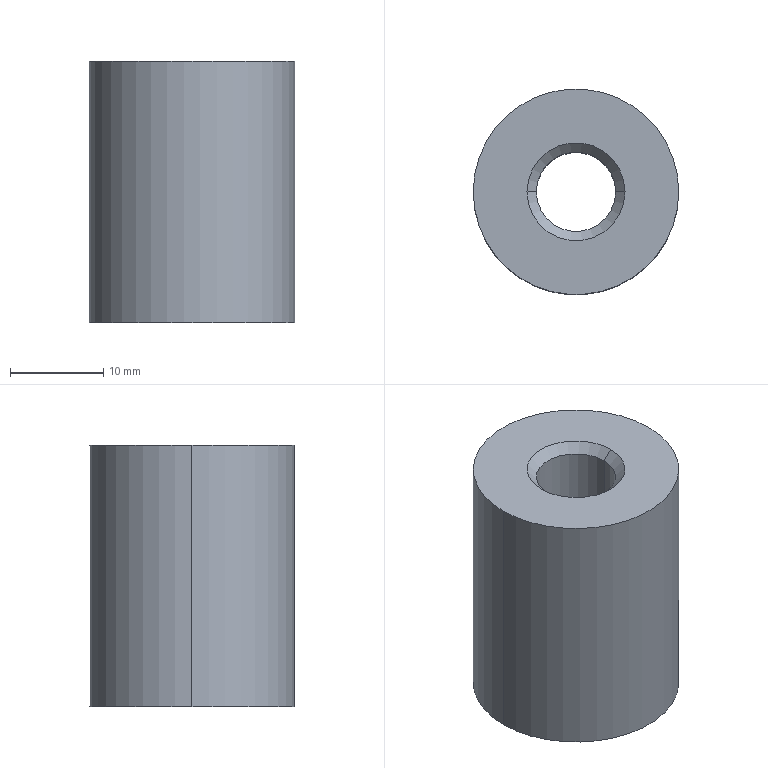Part | SolidWorks | features Chamfer 1, Extrusion 1, Helix 1, ICE 1 | 1 solid | 8 faces | box 22 x 22 x 28 mm | volume 9040 mm3 | cylinder 4 | cone 2 | plane 2 | commonest cylinder face diameters 8.5 x2 22 x2
STEP:
#1=CARTESIAN_POINT('',(-4.25,0.,27.));
#2=VERTEX_POINT('',#1);
#3=CARTESIAN_POINT('',(4.25,0.,27.));
#4=VERTEX_POINT('',#3);
#5=CARTESIAN_POINT('',(0.,0.,27.));
#6=DIRECTION('',(0.,0.,1.));
#7=DIRECTION('',(1.,0.,0.));
#8=AXIS2_PLACEMENT_3D('',#5,#6,#7);
#9=CIRCLE('',#8,4.25);
#10=EDGE_CURVE('',#2,#4,#9,.T.);
#11=ORIENTED_EDGE('',*,*,#10,.F.);
#12=CARTESIAN_POINT('',(-5.25,0.,28.));
#13=VERTEX_POINT('',#12);
#14=CARTESIAN_POINT('',(-4.25,0.,27.));
#15=DIRECTION('',(-0.7071,0.,0.7071));
#16=VECTOR('',#15,1000.);
#17=LINE('',#14,#16);
#18=EDGE_CURVE('',#2,#13,#17,.T.);
#19=ORIENTED_EDGE('',*,*,#18,.T.);
#20=CARTESIAN_POINT('',(5.25,0.,28.));
#21=VERTEX_POINT('',#20);
#22=CARTESIAN_POINT('',(0.,0.,28.));
#23=DIRECTION('',(0.,0.,-1.));
#24=DIRECTION('',(1.,0.,0.));
#25=AXIS2_PLACEMENT_3D('',#22,#23,#24);
#26=CIRCLE('',#25,5.25);
#27=EDGE_CURVE('',#21,#13,#26,.T.);
#28=ORIENTED_EDGE('',*,*,#27,.F.);
#29=CARTESIAN_POINT('',(4.25,0.,27.));
#30=DIRECTION('',(0.7071,0.,0.7071));
#31=VECTOR('',#30,1000.);
#32=LINE('',#29,#31);
#33=EDGE_CURVE('',#4,#21,#32,.T.);
#34=ORIENTED_EDGE('',*,*,#33,.F.);
#35=EDGE_LOOP('',(#11,#19,#28,#34));
#36=FACE_OUTER_BOUND('',#35,.T.);
#37=CARTESIAN_POINT('',(0.,0.,27.));
#38=DIRECTION('',(0.,0.,1.));
#39=DIRECTION('',(1.,0.,0.));
#40=AXIS2_PLACEMENT_3D('',#37,#38,#39);
#41=CONICAL_SURFACE('',#40,4.25,0.7854);
#42=ADVANCED_FACE('',(#36),#41,.F.);
#43=CARTESIAN_POINT('',(-4.25,0.,0.));
#44=VERTEX_POINT('',#43);
#45=CARTESIAN_POINT('',(4.25,0.,0.));
#46=VERTEX_POINT('',#45);
#47=CARTESIAN_POINT('',(0.,0.,0.));
#48=DIRECTION('',(0.,0.,1.));
#49=DIRECTION('',(1.,0.,0.));
#50=AXIS2_PLACEMENT_3D('',#47,#48,#49);
#51=CIRCLE('',#50,4.25);
#52=EDGE_CURVE('',#44,#46,#51,.T.);
#53=ORIENTED_EDGE('',*,*,#52,.F.);
#54=CARTESIAN_POINT('',(-4.25,0.,-10.));
#55=DIRECTION('',(0.,0.,1.));
#56=VECTOR('',#55,1000.);
#57=LINE('',#54,#56);
#58=EDGE_CURVE('',#44,#2,#57,.T.);
#59=ORIENTED_EDGE('',*,*,#58,.T.);
#60=ORIENTED_EDGE('',*,*,#10,.T.);
#61=CARTESIAN_POINT('',(4.25,0.,-10.));
#62=DIRECTION('',(0.,0.,1.));
#63=VECTOR('',#62,1000.);
#64=LINE('',#61,#63);
#65=EDGE_CURVE('',#46,#4,#64,.T.);
#66=ORIENTED_EDGE('',*,*,#65,.F.);
#67=EDGE_LOOP('',(#53,#59,#60,#66));
#68=FACE_OUTER_BOUND('',#67,.T.);
#69=CARTESIAN_POINT('',(0.,0.,-10.));
#70=DIRECTION('',(0.,0.,1.));
#71=DIRECTION('',(1.,0.,0.));
#72=AXIS2_PLACEMENT_3D('',#69,#70,#71);
#73=CYLINDRICAL_SURFACE('',#72,4.25);
#74=ADVANCED_FACE('',(#68),#73,.F.);
#75=CARTESIAN_POINT('',(11.,0.,28.));
#76=VERTEX_POINT('',#75);
#77=CARTESIAN_POINT('',(-11.,0.,28.));
#78=VERTEX_POINT('',#77);
#79=CARTESIAN_POINT('',(0.,0.,28.));
#80=DIRECTION('',(0.,0.,1.));
#81=DIRECTION('',(1.,0.,0.));
#82=AXIS2_PLACEMENT_3D('',#79,#80,#81);
#83=CIRCLE('',#82,11.);
#84=EDGE_CURVE('',#76,#78,#83,.T.);
#85=ORIENTED_EDGE('',*,*,#84,.F.);
#86=CARTESIAN_POINT('',(11.,0.,0.));
#87=VERTEX_POINT('',#86);
#88=CARTESIAN_POINT('',(11.,0.,28.));
#89=DIRECTION('',(0.,0.,-1.));
#90=VECTOR('',#89,1000.);
#91=LINE('',#88,#90);
#92=EDGE_CURVE('',#76,#87,#91,.T.);
#93=ORIENTED_EDGE('',*,*,#92,.T.);
#94=CARTESIAN_POINT('',(-11.,0.,0.));
#95=VERTEX_POINT('',#94);
#96=CARTESIAN_POINT('',(0.,0.,0.));
#97=DIRECTION('',(0.,0.,1.));
#98=DIRECTION('',(1.,0.,0.));
#99=AXIS2_PLACEMENT_3D('',#96,#97,#98);
#100=CIRCLE('',#99,11.);
#101=EDGE_CURVE('',#87,#95,#100,.T.);
#102=ORIENTED_EDGE('',*,*,#101,.T.);
#103=CARTESIAN_POINT('',(-11.,0.,28.));
#104=DIRECTION('',(0.,0.,-1.));
#105=VECTOR('',#104,1000.);
#106=LINE('',#103,#105);
#107=EDGE_CURVE('',#78,#95,#106,.T.);
#108=ORIENTED_EDGE('',*,*,#107,.F.);
#109=EDGE_LOOP('',(#85,#93,#102,#108));
#110=FACE_OUTER_BOUND('',#109,.T.);
#111=CARTESIAN_POINT('',(0.,0.,28.));
#112=DIRECTION('',(0.,0.,-1.));
#113=DIRECTION('',(-1.,0.,0.));
#114=AXIS2_PLACEMENT_3D('',#111,#112,#113);
#115=CYLINDRICAL_SURFACE('',#114,11.);
#116=ADVANCED_FACE('',(#110),#115,.T.);
#117=ORIENTED_EDGE('',*,*,#92,.F.);
#118=CARTESIAN_POINT('',(0.,0.,28.));
#119=DIRECTION('',(0.,0.,1.));
#120=DIRECTION('',(1.,0.,0.));
#121=AXIS2_PLACEMENT_3D('',#118,#119,#120);
#122=CIRCLE('',#121,11.);
#123=EDGE_CURVE('',#78,#76,#122,.T.);
#124=ORIENTED_EDGE('',*,*,#123,.F.);
#125=ORIENTED_EDGE('',*,*,#107,.T.);
#126=CARTESIAN_POINT('',(0.,0.,0.));
#127=DIRECTION('',(0.,0.,1.));
#128=DIRECTION('',(1.,0.,0.));
#129=AXIS2_PLACEMENT_3D('',#126,#127,#128);
#130=CIRCLE('',#129,11.);
#131=EDGE_CURVE('',#95,#87,#130,.T.);
#132=ORIENTED_EDGE('',*,*,#131,.T.);
#133=EDGE_LOOP('',(#117,#124,#125,#132));
#134=FACE_OUTER_BOUND('',#133,.T.);
#135=CARTESIAN_POINT('',(0.,0.,28.));
#136=DIRECTION('',(0.,0.,-1.));
#137=DIRECTION('',(-1.,0.,0.));
#138=AXIS2_PLACEMENT_3D('',#135,#136,#137);
#139=CYLINDRICAL_SURFACE('',#138,11.);
#140=ADVANCED_FACE('',(#134),#139,.T.);
#141=ORIENTED_EDGE('',*,*,#27,.T.);
#142=CARTESIAN_POINT('',(0.,0.,28.));
#143=DIRECTION('',(0.,0.,-1.));
#144=DIRECTION('',(1.,0.,0.));
#145=AXIS2_PLACEMENT_3D('',#142,#143,#144);
#146=CIRCLE('',#145,5.25);
#147=EDGE_CURVE('',#13,#21,#146,.T.);
#148=ORIENTED_EDGE('',*,*,#147,.T.);
#149=EDGE_LOOP('',(#141,#148));
#150=FACE_BOUND('',#149,.T.);
#151=ORIENTED_EDGE('',*,*,#123,.T.);
#152=ORIENTED_EDGE('',*,*,#84,.T.);
#153=EDGE_LOOP('',(#151,#152));
#154=FACE_OUTER_BOUND('',#153,.T.);
#155=CARTESIAN_POINT('',(0.,0.,28.));
#156=DIRECTION('',(0.,0.,1.));
#157=DIRECTION('',(1.,0.,0.));
#158=AXIS2_PLACEMENT_3D('',#155,#156,#157);
#159=PLANE('',#158);
#160=ADVANCED_FACE('',(#150,#154),#159,.T.);
#161=CARTESIAN_POINT('',(0.,0.,0.));
#162=DIRECTION('',(0.,0.,1.));
#163=DIRECTION('',(1.,0.,0.));
#164=AXIS2_PLACEMENT_3D('',#161,#162,#163);
#165=CIRCLE('',#164,4.25);
#166=EDGE_CURVE('',#46,#44,#165,.T.);
#167=ORIENTED_EDGE('',*,*,#166,.T.);
#168=ORIENTED_EDGE('',*,*,#52,.T.);
#169=EDGE_LOOP('',(#167,#168));
#170=FACE_BOUND('',#169,.T.);
#171=ORIENTED_EDGE('',*,*,#131,.F.);
#172=ORIENTED_EDGE('',*,*,#101,.F.);
#173=EDGE_LOOP('',(#171,#172));
#174=FACE_OUTER_BOUND('',#173,.T.);
#175=CARTESIAN_POINT('',(0.,0.,0.));
#176=DIRECTION('',(0.,0.,1.));
#177=DIRECTION('',(1.,0.,0.));
#178=AXIS2_PLACEMENT_3D('',#175,#176,#177);
#179=PLANE('',#178);
#180=ADVANCED_FACE('',(#170,#174),#179,.F.);
#181=ORIENTED_EDGE('',*,*,#58,.F.);
#182=ORIENTED_EDGE('',*,*,#166,.F.);
#183=ORIENTED_EDGE('',*,*,#65,.T.);
#184=CARTESIAN_POINT('',(0.,0.,27.));
#185=DIRECTION('',(0.,0.,1.));
#186=DIRECTION('',(1.,0.,0.));
#187=AXIS2_PLACEMENT_3D('',#184,#185,#186);
#188=CIRCLE('',#187,4.25);
#189=EDGE_CURVE('',#4,#2,#188,.T.);
#190=ORIENTED_EDGE('',*,*,#189,.T.);
#191=EDGE_LOOP('',(#181,#182,#183,#190));
#192=FACE_OUTER_BOUND('',#191,.T.);
#193=CARTESIAN_POINT('',(0.,0.,-10.));
#194=DIRECTION('',(0.,0.,1.));
#195=DIRECTION('',(1.,0.,0.));
#196=AXIS2_PLACEMENT_3D('',#193,#194,#195);
#197=CYLINDRICAL_SURFACE('',#196,4.25);
#198=ADVANCED_FACE('',(#192),#197,.F.);
#199=ORIENTED_EDGE('',*,*,#18,.F.);
#200=ORIENTED_EDGE('',*,*,#189,.F.);
#201=ORIENTED_EDGE('',*,*,#33,.T.);
#202=ORIENTED_EDGE('',*,*,#147,.F.);
#203=EDGE_LOOP('',(#199,#200,#201,#202));
#204=FACE_OUTER_BOUND('',#203,.T.);
#205=CARTESIAN_POINT('',(0.,0.,27.));
#206=DIRECTION('',(0.,0.,1.));
#207=DIRECTION('',(1.,0.,0.));
#208=AXIS2_PLACEMENT_3D('',#205,#206,#207);
#209=CONICAL_SURFACE('',#208,4.25,0.7854);
#210=ADVANCED_FACE('',(#204),#209,.F.);
#211=CLOSED_SHELL('',(#42,#74,#116,#140,#160,#180,#198,#210));
#212=MANIFOLD_SOLID_BREP('',#211);
#213=CARTESIAN_POINT('',(0.,0.,0.));
#214=DIRECTION('',(0.,0.,1.));
#215=DIRECTION('',(1.,0.,0.));
#216=AXIS2_PLACEMENT_3D('',#213,#214,#215);
#217=(LENGTH_UNIT()NAMED_UNIT(*)SI_UNIT(.MILLI.,.METRE.));
#218=UNCERTAINTY_MEASURE_WITH_UNIT(LENGTH_MEASURE(0.00001),#217,'','');
#219=(NAMED_UNIT(*)PLANE_ANGLE_UNIT()SI_UNIT($,.RADIAN.));
#220=(NAMED_UNIT(*)SI_UNIT($,.STERADIAN.)SOLID_ANGLE_UNIT());
#221=(GEOMETRIC_REPRESENTATION_CONTEXT(3)GLOBAL_UNCERTAINTY_ASSIGNED_CONTEXT((#218))GLOBAL_UNIT_ASSIGNED_CONTEXT((#217,#219,#220))REPRESENTATION_CONTEXT('',''));
#222=ADVANCED_BREP_SHAPE_REPRESENTATION('',(#212,#216),#221);